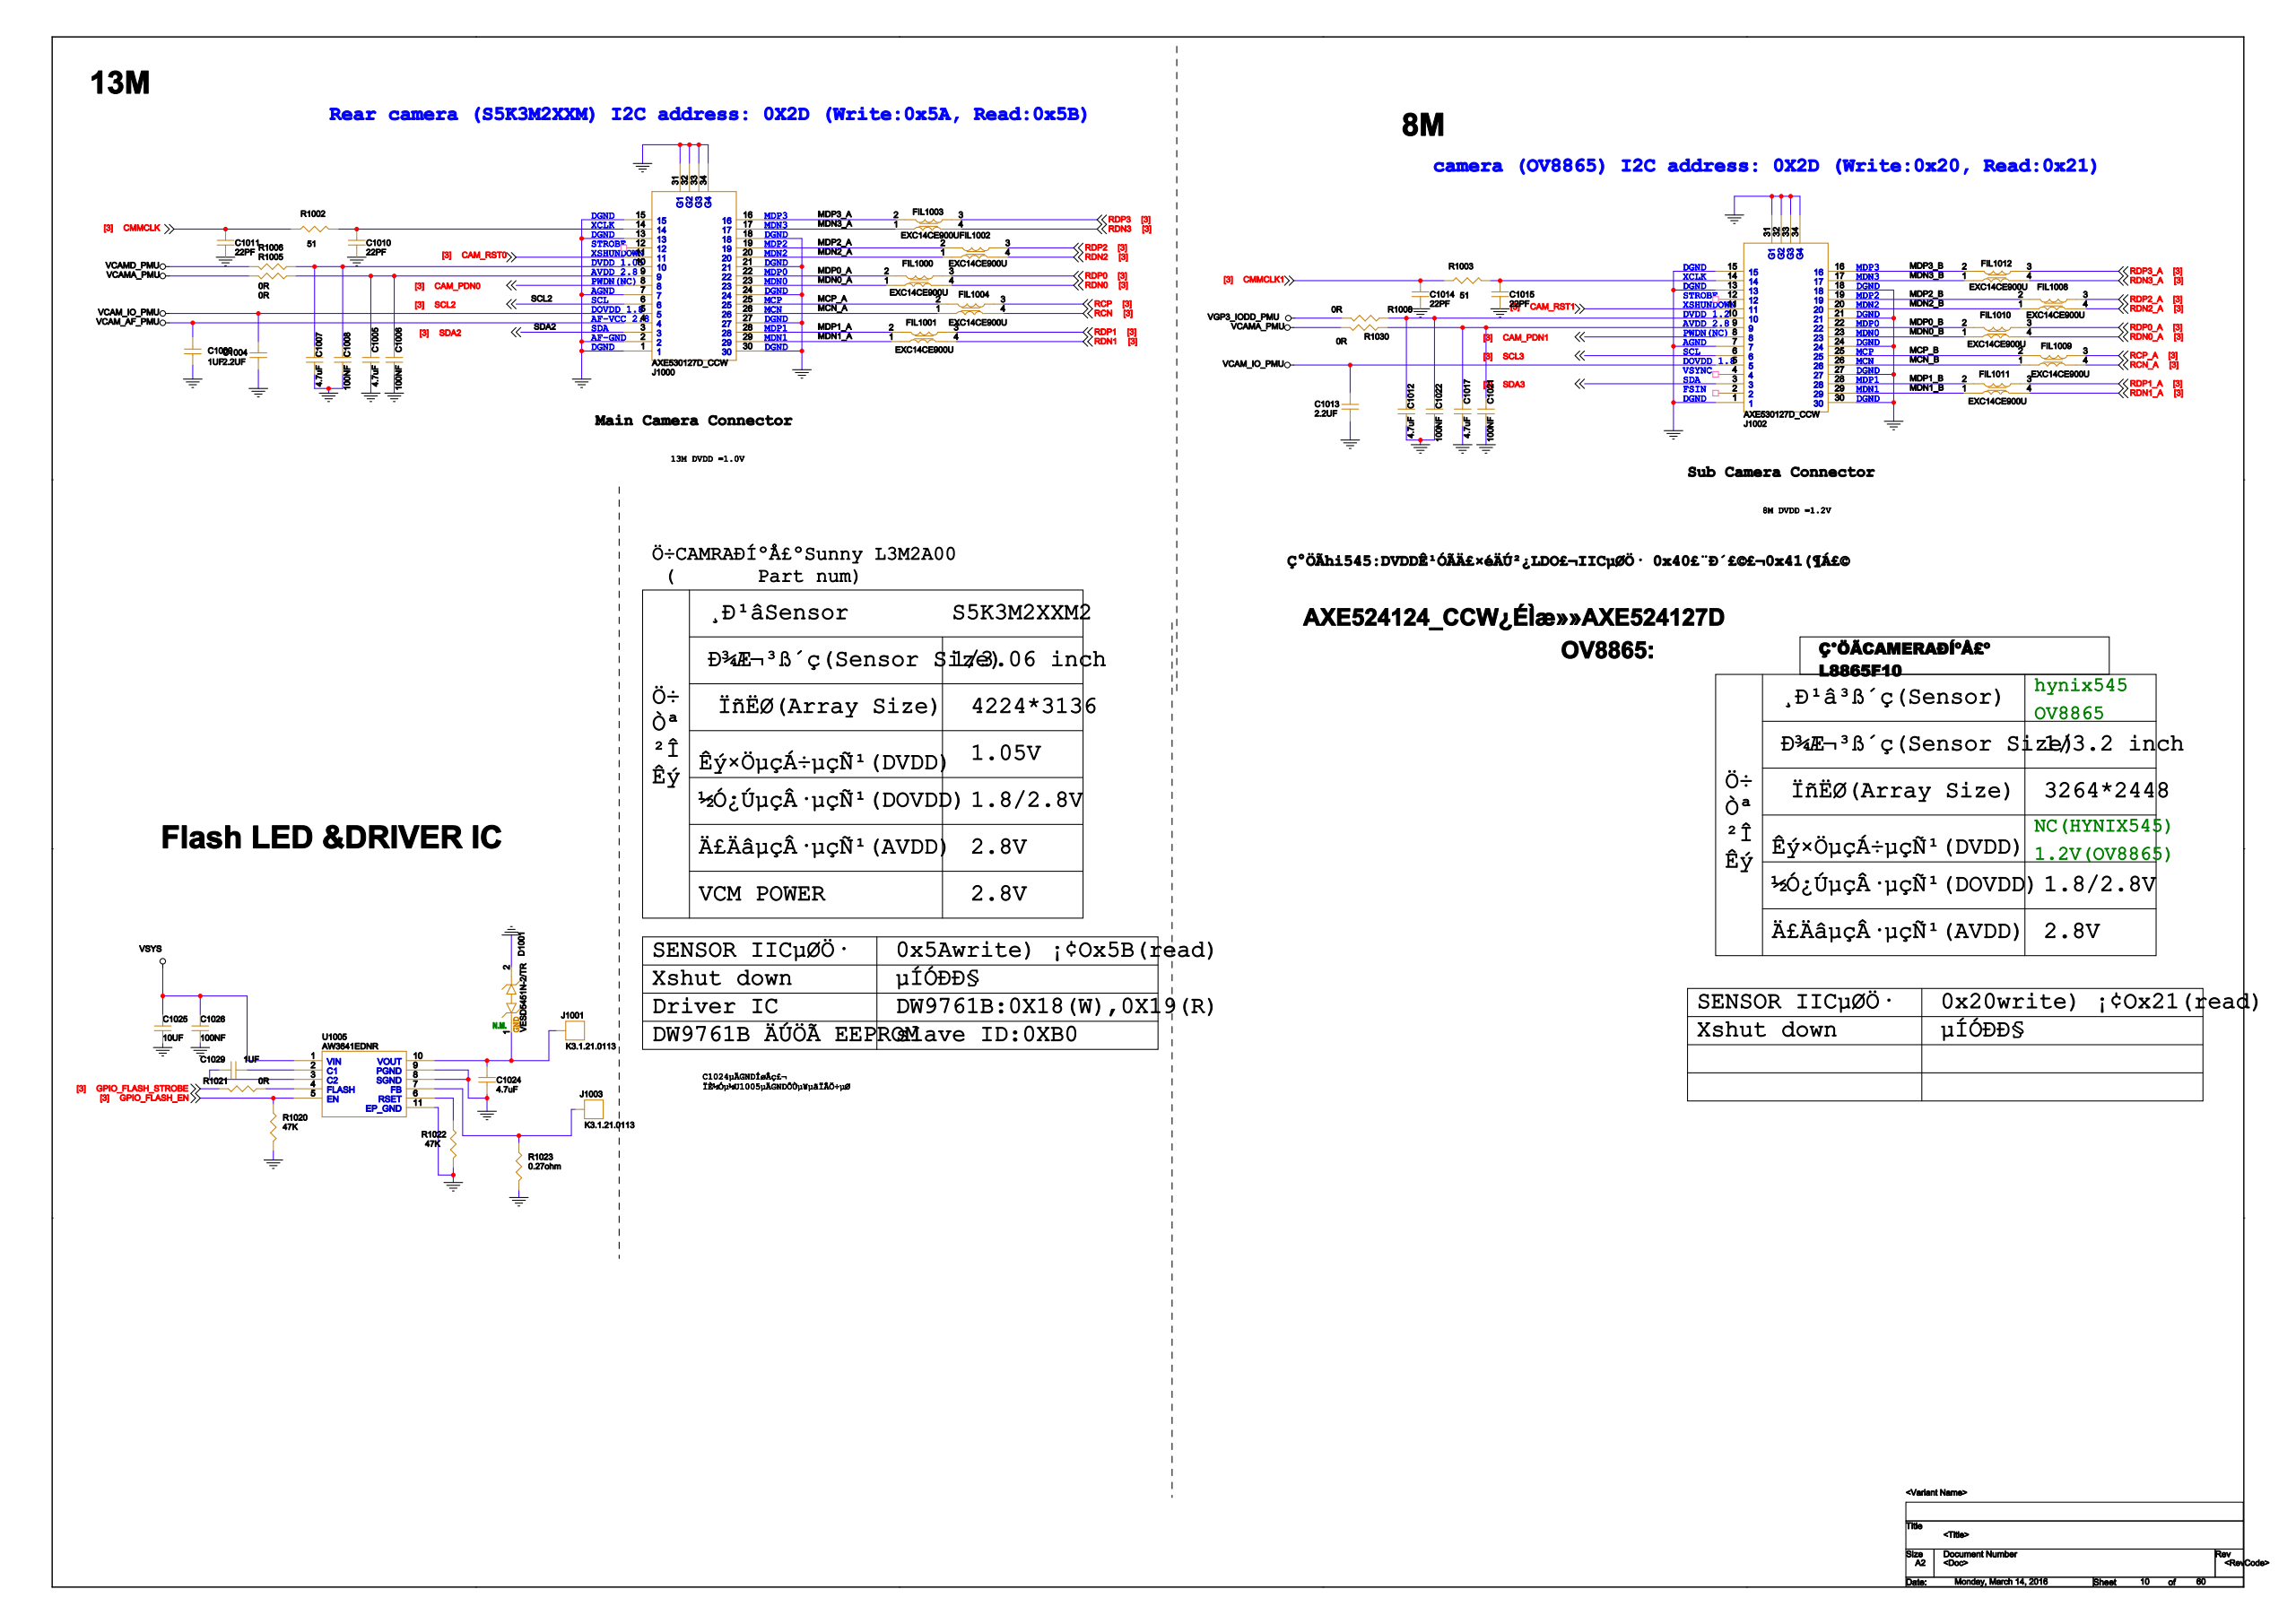Circuit board | Cadence Allegro | 1088 parts | 793 nets | one sheet of the schematic
Parts on this sheet (reference | value | footprint):
C1000 | 1UF | C0201
C1004 | 2.2UF | 0402-BIG
C1005 | 4.7uF | 0402-BIG
C1006 | 100NF | C0201
C1007 | 4.7uF | 0402-BIG
C1008 | 100NF | C0201
C1010 | 22PF | C0201
C1011 | 22PF | C0201
C1012 | 4.7uF | 0402-BIG
C1013 | 2.2UF | 0402-BIG
C1014 | 22PF | C0201
C1015 | 22PF | C0201
C1017 | 4.7uF | 0402-BIG
C1021 | 100NF | C0201
C1022 | 100NF | C0201
C1024 | 4.7uF | 0402-BIG
C1025 | 10UF | 0402-BIG
C1026 | 100NF | C0201
C1029 | 1UF | C0201
D1001
FIL1000 | EXC14CE900U | EXC14CE900U
FIL1001 | EXC14CE900U | EXC14CE900U
FIL1002 | EXC14CE900U | EXC14CE900U
FIL1003 | EXC14CE900U | EXC14CE900U
FIL1004 | EXC14CE900U | EXC14CE900U
FIL1008 | EXC14CE900U | EXC14CE900U
FIL1009 | EXC14CE900U | EXC14CE900U
FIL1010 | EXC14CE900U | EXC14CE900U
FIL1011 | EXC14CE900U | EXC14CE900U
FIL1012 | EXC14CE900U | EXC14CE900U
J1000 | AXE530127D_CCW | BTB_AXE530124_CCW
J1001 | K3.1.21.0113 | PIN_ANT_K3_1_21_0113
J1002 | AXE530127D_CCW | BTB_AXE530124_CCW
J1003 | K3.1.21.0113 | PIN_ANT_K3_1_21_0113
R1002 | 51 | R0201
R1003 | 51 | R0201
R1005 | 0R | R0201
R1006 | 0R | R0201
R1008 | 0R | R0201
R1020 | 47K | R0201
R1021 | 0R | R0201
R1022 | 47K | R0201
R1023 | 0.27ohm | R0805
R1030 | 0R | R0201
U1005 | AW3641EDNR | DFN10_3X3X0P9_0P5
Nets of these parts (net: part-pin ...):
GND: C1000-1 C1004-2 C1005-2 C1006-2 C1007-2 C1008-2 C1010-2 C1011-2 C1012-2 C1013-2 C1014-2 C1015-2 C1017-2 C1021-2 C1022-2 C1024-2 C1025-2 C1026-2 D1001-2 R1020-2 R1022-2 R1023-2 U1005-8 U1005-9 U1005-11 J1000-1 J1000-2 J1000-7 J1000-13 J1000-15 J1000-18 J1000-21 J1000-24 J1000-27 J1000-30 J1000-31 J1000-32 J1000-33 J1000-34 J1002-1 J1002-7 J1002-13 J1002-15 J1002-18 J1002-21 J1002-24 J1002-27 J1002-30 J1002-31 J1002-32 J1002-33 J1002-34
VSYS: C1025-1 C1026-1 U1005-1
CMMCLK: C1011-1 R1002-1
CMMCLK1: C1014-1 R1003-1
CAM_PDN0: J1000-8
CAM_PDN1: J1002-8
CAM_RST0: J1000-11
CAM_RST1: J1002-11
RCN: FIL1004-4
RCN_A: FIL1009-4
RCP: FIL1004-3
RCP_A: FIL1009-3
RDN0: FIL1000-4
RDN0_A: FIL1010-4
RDN1: FIL1001-4
RDN1_A: FIL1011-4
RDN2: FIL1002-4
RDN2_A: FIL1008-4
RDN3: FIL1003-4
RDN3_A: FIL1012-4
RDP0: FIL1000-3
RDP0_A: FIL1010-3
RDP1: FIL1001-3
RDP1_A: FIL1011-3
RDP2: FIL1002-3
RDP2_A: FIL1008-3
RDP3: FIL1003-3
RDP3_A: FIL1012-3
GPIO_FLASH_EN: R1020-1 U1005-5
GPIO_FLASH_STROBE: R1021-2
SCL2: J1000-6
SCL3: J1002-6
SDA2: J1000-3
SDA3: J1002-3
N34218924: J1003-1 R1023-1 U1005-7
N34218574: C1024-1 D1001-1 J1001-1 U1005-10
MDN0_A: FIL1000-1 J1000-23
MDP0_A: FIL1000-2 J1000-22
MDN1_A: FIL1001-1 J1000-29
MDP1_A: FIL1001-2 J1000-28
MDN2_A: FIL1002-1 J1000-20
MDP2_A: FIL1002-2 J1000-19
MDN3_A: FIL1003-1 J1000-17
MDP3_A: FIL1003-2 J1000-16
MCN_A: FIL1004-1 J1000-26
MCP_A: FIL1004-2 J1000-25
MDN2_B: FIL1008-1 J1002-20
MDP2_B: FIL1008-2 J1002-19
MCN_B: FIL1009-1 J1002-26
MCP_B: FIL1009-2 J1002-25
MDN0_B: FIL1010-1 J1002-23
MDP0_B: FIL1010-2 J1002-22
MDN1_B: FIL1011-1 J1002-29
MDP1_B: FIL1011-2 J1002-28
MDN3_B: FIL1012-1 J1002-17
MDP3_B: FIL1012-2 J1002-16
N34217211: C1029-1 U1005-2
N34217229: C1029-2 U1005-3
N41686647: R1021-1 U1005-4
N34218917: R1022-1 U1005-6
VCAM_AF_PMU: C1000-2 J1000-4
VCAMA_PMU: R1005-2 R1030-2
VCAM_IO_PMU: C1004-1 C1013-1 J1000-5 J1002-5
VGP3_IODD_PMU: R1008-2
N33140582: C1005-1 C1006-1 R1005-1 J1000-9
N33143712: C1007-1 C1008-1 R1006-1 J1000-10
N33734200: C1012-1 C1022-1 R1008-1 J1002-10
N33734083: C1017-1 C1021-1 R1030-1 J1002-9
N33138858: C1010-1 R1002-2 J1000-14
N33733853: C1015-1 R1003-2 J1002-14
VCAMD_PMU: R1006-2